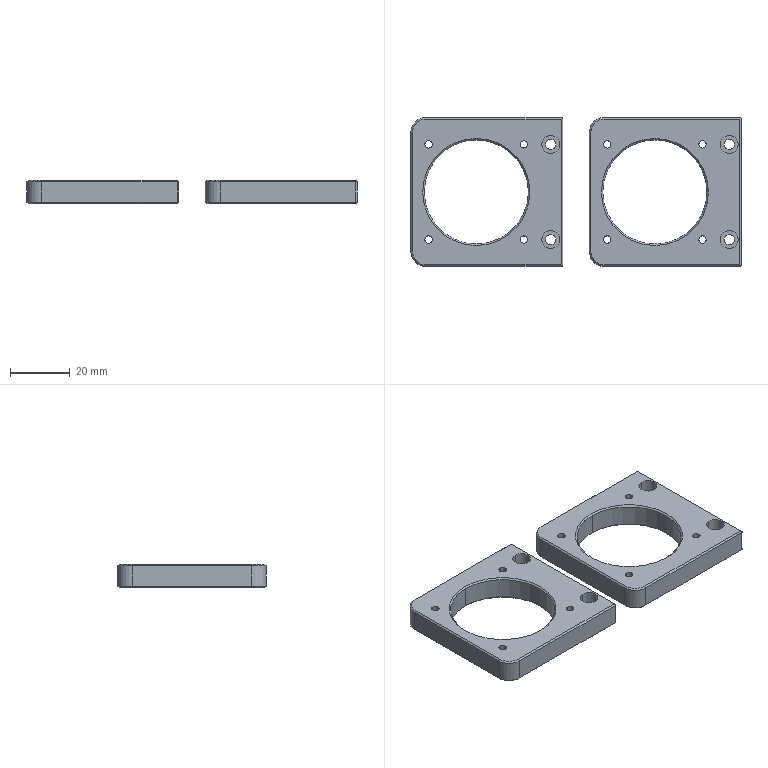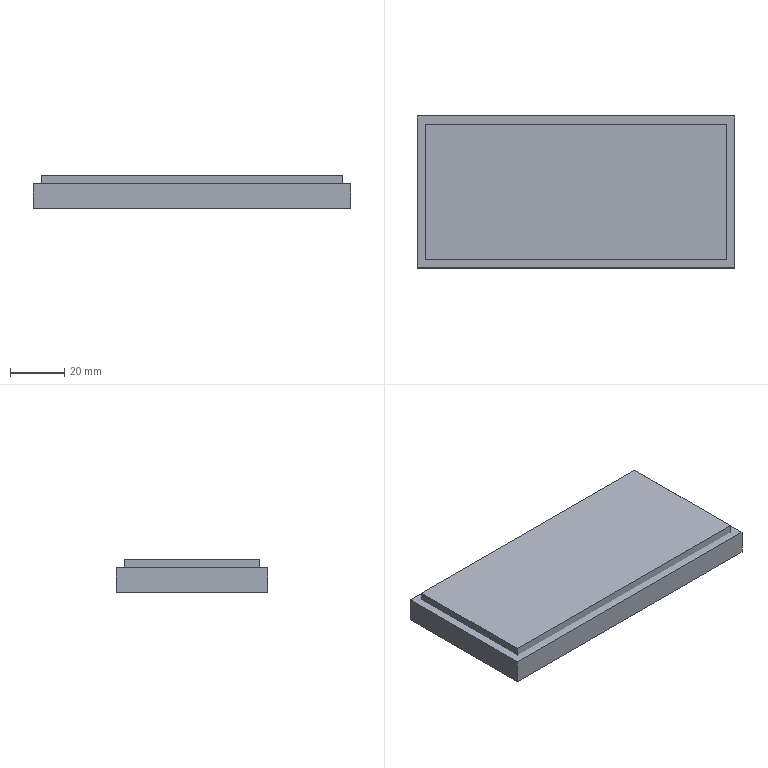CAM job | NX | 3-axis milling, drilling | part box 111 x 50 x 8 mm | stock box 117 x 56 x 12 mm
Tools:
number,name,description,diameter,corner_radius,flute_length,length,flutes
1,D63,Milling Tool-5 Parameters,63.0,0.0,50.0,75.0,2
2,D4A45,Milling Tool-5 Parameters,4.0,0.0,2.0,2.0,2
6,D6,Milling Tool-5 Parameters,6.0,0.0,50.0,75.0,2
15,3.5ZT,Drilling Tool,3.5,0.0,35.0,50.0,2
12,2.5ZT,Drilling Tool,2.5,0.0,35.0,50.0,2
4,D4,Milling Tool-5 Parameters,4.0,0.0,50.0,75.0,2
Operations:
program,operation,operation_type,tool,method,geometry_group,spindle_rpm,surface_speed,feed_per_tooth,feed_cut,feed_plunge,cut_length_mm,path_length_mm,cut_time_min,machine_time_min
1虎钳,FLOOR_WALL,VolumeBased25DMillingOperation,D63,METHOD,A,6500.0,1286.0,0.0962,1250.0,100.0,192.0,246.0,0.1536,0.159
1虎钳,DRILLING_COPY,Operation,D4A45,METHOD,A,5000.0,62.0,0.025,250.0,0.0,56.0,475.141,0.224,0.2659
1虎钳,DRILLING_COPY_COPY_COPY_COPY_COPY,Operation,2.5ZT,METHOD,A,1910.0,21.0,0.0471,180.0,0.0,106.009,510.039,0.5889,0.6293
1虎钳,DRILLING_COPY_COPY_COPY_COPY_COPY_COPY,Operation,3.5ZT,METHOD,A,1910.0,21.0,0.0471,180.0,0.0,52.206,305.759,0.29,0.3154
1虎钳,ZLEVEL_PROFILE_1_COPY_1_COPY_COPY,ZLevelMilling,D4A45,METHOD,A,9500.0,179.0,0.0526,1000.0,100.0,743.898,2300.269,0.7439,0.8995
1虎钳,ZLEVEL_PROFILE_COPY_COPY_1_COPY,ZLevelMilling,D6,METHOD,A,9500.0,179.0,0.1158,2200.0,1000.0,7073.052,7318.095,3.257,3.281
1虎钳,HOLE_MILLING_COPY,CylinderMilling,D6,METHOD,A,9496.0,179.0,0.1158,2200.0,100.0,3961.317,4156.317,1.801,1.82
1虎钳,ZLEVEL_PROFILE_COPY_COPY_COPY_COPY_COPY,ZLevelMilling,D4,MILL_FINISH,A,9500.0,119.0,0.0632,1200.0,1000.0,630.707,1075.25,0.5269,0.5714
1虎钳,HOLE_MILLING,CylinderMilling,D4,METHOD,A,9500.0,179.0,0.0789,1500.0,100.0,352.494,740.494,0.235,0.2738
2,FLOOR_WALL_COPY,VolumeBased25DMillingOperation,D63,METHOD,B,6500.0,1286.0,0.0962,1250.0,100.0,744.0,1488.001,0.5952,0.6696
2,ZLEVEL_PROFILE_1_COPY_1_COPY_COPY_COPY,ZLevelMilling,D4A45,METHOD,B,9500.0,179.0,0.0526,1000.0,100.0,705.057,2111.174,0.7051,0.8457